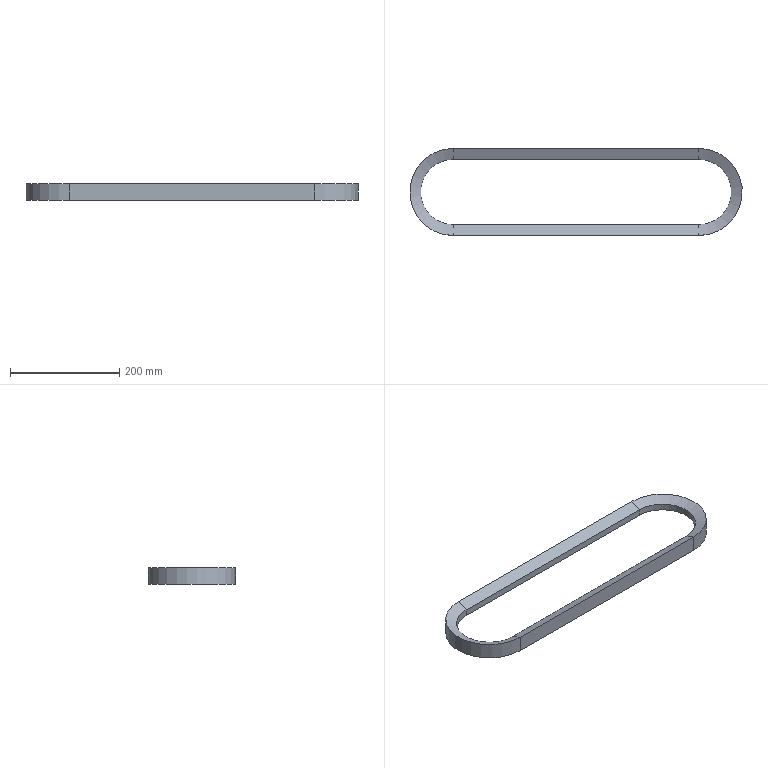Part | NX | 1 solid | 16 faces | box 610 x 160 x 30 mm | volume 573090 mm3 | plane 8 | cylinder 4 | cone 4 | commonest cylinder face diameters 120 x2 160 x2
STEP:
#1=CARTESIAN_POINT('',(450.,-80.,-15.));
#2=VERTEX_POINT('',#1);
#3=CARTESIAN_POINT('',(450.,-80.,15.));
#4=VERTEX_POINT('',#3);
#5=CARTESIAN_POINT('',(450.,-80.,-15.));
#6=DIRECTION('',(0.,0.,1.));
#7=VECTOR('',#6,1.);
#8=LINE('',#5,#7);
#9=EDGE_CURVE('',#2,#4,#8,.T.);
#10=ORIENTED_EDGE('',*,*,#9,.F.);
#11=CARTESIAN_POINT('',(450.,80.,-15.));
#12=VERTEX_POINT('',#11);
#13=CARTESIAN_POINT('',(450.,0.,-15.));
#14=DIRECTION('',(0.,0.,1.));
#15=DIRECTION('',(1.,0.,0.));
#16=AXIS2_PLACEMENT_3D('',#13,#14,#15);
#17=CIRCLE('',#16,80.);
#18=EDGE_CURVE('',#2,#12,#17,.T.);
#19=ORIENTED_EDGE('',*,*,#18,.T.);
#20=CARTESIAN_POINT('',(450.,80.,15.));
#21=VERTEX_POINT('',#20);
#22=CARTESIAN_POINT('',(450.,80.,-15.));
#23=DIRECTION('',(0.,0.,1.));
#24=VECTOR('',#23,1.);
#25=LINE('',#22,#24);
#26=EDGE_CURVE('',#12,#21,#25,.T.);
#27=ORIENTED_EDGE('',*,*,#26,.T.);
#28=CARTESIAN_POINT('',(450.,0.,15.));
#29=DIRECTION('',(0.,0.,1.));
#30=DIRECTION('',(1.,0.,0.));
#31=AXIS2_PLACEMENT_3D('',#28,#29,#30);
#32=CIRCLE('',#31,80.);
#33=EDGE_CURVE('',#4,#21,#32,.T.);
#34=ORIENTED_EDGE('',*,*,#33,.F.);
#35=EDGE_LOOP('',(#10,#19,#27,#34));
#36=FACE_OUTER_BOUND('',#35,.T.);
#37=CARTESIAN_POINT('',(450.,0.,0.));
#38=DIRECTION('',(0.,0.,1.));
#39=DIRECTION('',(1.,0.,0.));
#40=AXIS2_PLACEMENT_3D('',#37,#38,#39);
#41=CYLINDRICAL_SURFACE('',#40,80.);
#42=ADVANCED_FACE('',(#36),#41,.T.);
#43=CARTESIAN_POINT('',(450.,-60.,-6.25));
#44=VERTEX_POINT('',#43);
#45=CARTESIAN_POINT('',(450.,-60.,-6.25));
#46=DIRECTION('',(0.,-0.9162,-0.4008));
#47=VECTOR('',#46,1.);
#48=LINE('',#45,#47);
#49=EDGE_CURVE('',#44,#2,#48,.T.);
#50=ORIENTED_EDGE('',*,*,#49,.F.);
#51=CARTESIAN_POINT('',(450.,60.,-6.25));
#52=VERTEX_POINT('',#51);
#53=CARTESIAN_POINT('',(450.,0.,-6.25));
#54=DIRECTION('',(0.,0.,1.));
#55=DIRECTION('',(1.,0.,0.));
#56=AXIS2_PLACEMENT_3D('',#53,#54,#55);
#57=CIRCLE('',#56,60.);
#58=EDGE_CURVE('',#44,#52,#57,.T.);
#59=ORIENTED_EDGE('',*,*,#58,.T.);
#60=CARTESIAN_POINT('',(450.,60.,-6.25));
#61=DIRECTION('',(0.,0.9162,-0.4008));
#62=VECTOR('',#61,1.);
#63=LINE('',#60,#62);
#64=EDGE_CURVE('',#52,#12,#63,.T.);
#65=ORIENTED_EDGE('',*,*,#64,.T.);
#66=ORIENTED_EDGE('',*,*,#18,.F.);
#67=EDGE_LOOP('',(#50,#59,#65,#66));
#68=FACE_OUTER_BOUND('',#67,.T.);
#69=CARTESIAN_POINT('',(450.,0.,-6.25));
#70=DIRECTION('',(0.,0.,-1.));
#71=DIRECTION('',(-1.,0.,0.));
#72=AXIS2_PLACEMENT_3D('',#69,#70,#71);
#73=CONICAL_SURFACE('',#72,60.,66.371);
#74=ADVANCED_FACE('',(#68),#73,.F.);
#75=CARTESIAN_POINT('',(450.,-60.,6.25));
#76=VERTEX_POINT('',#75);
#77=CARTESIAN_POINT('',(450.,-60.,6.25));
#78=DIRECTION('',(0.,0.,-1.));
#79=VECTOR('',#78,1.);
#80=LINE('',#77,#79);
#81=EDGE_CURVE('',#76,#44,#80,.T.);
#82=ORIENTED_EDGE('',*,*,#81,.F.);
#83=CARTESIAN_POINT('',(450.,60.,6.25));
#84=VERTEX_POINT('',#83);
#85=CARTESIAN_POINT('',(450.,0.,6.25));
#86=DIRECTION('',(0.,0.,1.));
#87=DIRECTION('',(1.,0.,0.));
#88=AXIS2_PLACEMENT_3D('',#85,#86,#87);
#89=CIRCLE('',#88,60.);
#90=EDGE_CURVE('',#76,#84,#89,.T.);
#91=ORIENTED_EDGE('',*,*,#90,.T.);
#92=CARTESIAN_POINT('',(450.,60.,6.25));
#93=DIRECTION('',(0.,0.,-1.));
#94=VECTOR('',#93,1.);
#95=LINE('',#92,#94);
#96=EDGE_CURVE('',#84,#52,#95,.T.);
#97=ORIENTED_EDGE('',*,*,#96,.T.);
#98=ORIENTED_EDGE('',*,*,#58,.F.);
#99=EDGE_LOOP('',(#82,#91,#97,#98));
#100=FACE_OUTER_BOUND('',#99,.T.);
#101=CARTESIAN_POINT('',(450.,0.,0.));
#102=DIRECTION('',(0.,0.,1.));
#103=DIRECTION('',(1.,0.,0.));
#104=AXIS2_PLACEMENT_3D('',#101,#102,#103);
#105=CYLINDRICAL_SURFACE('',#104,60.);
#106=ADVANCED_FACE('',(#100),#105,.F.);
#107=CARTESIAN_POINT('',(450.,-80.,15.));
#108=DIRECTION('',(0.,0.9162,-0.4008));
#109=VECTOR('',#108,1.);
#110=LINE('',#107,#109);
#111=EDGE_CURVE('',#4,#76,#110,.T.);
#112=ORIENTED_EDGE('',*,*,#111,.F.);
#113=ORIENTED_EDGE('',*,*,#33,.T.);
#114=CARTESIAN_POINT('',(450.,80.,15.));
#115=DIRECTION('',(0.,-0.9162,-0.4008));
#116=VECTOR('',#115,1.);
#117=LINE('',#114,#116);
#118=EDGE_CURVE('',#21,#84,#117,.T.);
#119=ORIENTED_EDGE('',*,*,#118,.T.);
#120=ORIENTED_EDGE('',*,*,#90,.F.);
#121=EDGE_LOOP('',(#112,#113,#119,#120));
#122=FACE_OUTER_BOUND('',#121,.T.);
#123=CARTESIAN_POINT('',(450.,0.,15.));
#124=DIRECTION('',(0.,0.,1.));
#125=DIRECTION('',(1.,0.,0.));
#126=AXIS2_PLACEMENT_3D('',#123,#124,#125);
#127=CONICAL_SURFACE('',#126,80.,66.371);
#128=ADVANCED_FACE('',(#122),#127,.F.);
#129=CARTESIAN_POINT('',(0.,-80.,-15.));
#130=VERTEX_POINT('',#129);
#131=CARTESIAN_POINT('',(0.,-80.,15.));
#132=VERTEX_POINT('',#131);
#133=CARTESIAN_POINT('',(0.,-80.,-15.));
#134=DIRECTION('',(0.,0.,1.));
#135=VECTOR('',#134,1.);
#136=LINE('',#133,#135);
#137=EDGE_CURVE('',#130,#132,#136,.T.);
#138=ORIENTED_EDGE('',*,*,#137,.F.);
#139=CARTESIAN_POINT('',(0.,-80.,-15.));
#140=DIRECTION('',(1.,0.,0.));
#141=VECTOR('',#140,1.);
#142=LINE('',#139,#141);
#143=EDGE_CURVE('',#130,#2,#142,.T.);
#144=ORIENTED_EDGE('',*,*,#143,.T.);
#145=ORIENTED_EDGE('',*,*,#9,.T.);
#146=CARTESIAN_POINT('',(0.,-80.,15.));
#147=DIRECTION('',(1.,0.,0.));
#148=VECTOR('',#147,1.);
#149=LINE('',#146,#148);
#150=EDGE_CURVE('',#132,#4,#149,.T.);
#151=ORIENTED_EDGE('',*,*,#150,.F.);
#152=EDGE_LOOP('',(#138,#144,#145,#151));
#153=FACE_OUTER_BOUND('',#152,.T.);
#154=CARTESIAN_POINT('',(0.,-80.,-15.));
#155=DIRECTION('',(0.,1.,0.));
#156=DIRECTION('',(0.,0.,1.));
#157=AXIS2_PLACEMENT_3D('',#154,#155,#156);
#158=PLANE('',#157);
#159=ADVANCED_FACE('',(#153),#158,.F.);
#160=CARTESIAN_POINT('',(0.,-60.,-6.25));
#161=VERTEX_POINT('',#160);
#162=CARTESIAN_POINT('',(0.,-60.,-6.25));
#163=DIRECTION('',(0.,-0.9162,-0.4008));
#164=VECTOR('',#163,1.);
#165=LINE('',#162,#164);
#166=EDGE_CURVE('',#161,#130,#165,.T.);
#167=ORIENTED_EDGE('',*,*,#166,.F.);
#168=CARTESIAN_POINT('',(0.,-60.,-6.25));
#169=DIRECTION('',(1.,0.,0.));
#170=VECTOR('',#169,1.);
#171=LINE('',#168,#170);
#172=EDGE_CURVE('',#161,#44,#171,.T.);
#173=ORIENTED_EDGE('',*,*,#172,.T.);
#174=ORIENTED_EDGE('',*,*,#49,.T.);
#175=ORIENTED_EDGE('',*,*,#143,.F.);
#176=EDGE_LOOP('',(#167,#173,#174,#175));
#177=FACE_OUTER_BOUND('',#176,.T.);
#178=CARTESIAN_POINT('',(0.,-60.,-6.25));
#179=DIRECTION('',(0.,-0.4008,0.9162));
#180=DIRECTION('',(0.,-0.9162,-0.4008));
#181=AXIS2_PLACEMENT_3D('',#178,#179,#180);
#182=PLANE('',#181);
#183=ADVANCED_FACE('',(#177),#182,.F.);
#184=CARTESIAN_POINT('',(0.,-60.,6.25));
#185=VERTEX_POINT('',#184);
#186=CARTESIAN_POINT('',(0.,-60.,6.25));
#187=DIRECTION('',(0.,0.,-1.));
#188=VECTOR('',#187,1.);
#189=LINE('',#186,#188);
#190=EDGE_CURVE('',#185,#161,#189,.T.);
#191=ORIENTED_EDGE('',*,*,#190,.F.);
#192=CARTESIAN_POINT('',(0.,-60.,6.25));
#193=DIRECTION('',(1.,0.,0.));
#194=VECTOR('',#193,1.);
#195=LINE('',#192,#194);
#196=EDGE_CURVE('',#185,#76,#195,.T.);
#197=ORIENTED_EDGE('',*,*,#196,.T.);
#198=ORIENTED_EDGE('',*,*,#81,.T.);
#199=ORIENTED_EDGE('',*,*,#172,.F.);
#200=EDGE_LOOP('',(#191,#197,#198,#199));
#201=FACE_OUTER_BOUND('',#200,.T.);
#202=CARTESIAN_POINT('',(0.,-60.,6.25));
#203=DIRECTION('',(0.,-1.,0.));
#204=DIRECTION('',(0.,0.,-1.));
#205=AXIS2_PLACEMENT_3D('',#202,#203,#204);
#206=PLANE('',#205);
#207=ADVANCED_FACE('',(#201),#206,.F.);
#208=CARTESIAN_POINT('',(0.,-80.,15.));
#209=DIRECTION('',(0.,0.9162,-0.4008));
#210=VECTOR('',#209,1.);
#211=LINE('',#208,#210);
#212=EDGE_CURVE('',#132,#185,#211,.T.);
#213=ORIENTED_EDGE('',*,*,#212,.F.);
#214=ORIENTED_EDGE('',*,*,#150,.T.);
#215=ORIENTED_EDGE('',*,*,#111,.T.);
#216=ORIENTED_EDGE('',*,*,#196,.F.);
#217=EDGE_LOOP('',(#213,#214,#215,#216));
#218=FACE_OUTER_BOUND('',#217,.T.);
#219=CARTESIAN_POINT('',(0.,-80.,15.));
#220=DIRECTION('',(0.,-0.4008,-0.9162));
#221=DIRECTION('',(0.,0.9162,-0.4008));
#222=AXIS2_PLACEMENT_3D('',#219,#220,#221);
#223=PLANE('',#222);
#224=ADVANCED_FACE('',(#218),#223,.F.);
#225=CARTESIAN_POINT('',(0.,60.,6.25));
#226=VERTEX_POINT('',#225);
#227=CARTESIAN_POINT('',(0.,0.,6.25));
#228=DIRECTION('',(0.,0.,-1.));
#229=DIRECTION('',(-1.,0.,0.));
#230=AXIS2_PLACEMENT_3D('',#227,#228,#229);
#231=CIRCLE('',#230,60.);
#232=EDGE_CURVE('',#185,#226,#231,.T.);
#233=ORIENTED_EDGE('',*,*,#232,.T.);
#234=CARTESIAN_POINT('',(0.,80.,15.));
#235=VERTEX_POINT('',#234);
#236=CARTESIAN_POINT('',(0.,80.,15.));
#237=DIRECTION('',(0.,-0.9162,-0.4008));
#238=VECTOR('',#237,1.);
#239=LINE('',#236,#238);
#240=EDGE_CURVE('',#235,#226,#239,.T.);
#241=ORIENTED_EDGE('',*,*,#240,.F.);
#242=CARTESIAN_POINT('',(0.,0.,15.));
#243=DIRECTION('',(0.,0.,-1.));
#244=DIRECTION('',(-1.,0.,0.));
#245=AXIS2_PLACEMENT_3D('',#242,#243,#244);
#246=CIRCLE('',#245,80.);
#247=EDGE_CURVE('',#132,#235,#246,.T.);
#248=ORIENTED_EDGE('',*,*,#247,.F.);
#249=ORIENTED_EDGE('',*,*,#212,.T.);
#250=EDGE_LOOP('',(#233,#241,#248,#249));
#251=FACE_OUTER_BOUND('',#250,.T.);
#252=CARTESIAN_POINT('',(0.,0.,15.));
#253=DIRECTION('',(0.,0.,1.));
#254=DIRECTION('',(1.,0.,0.));
#255=AXIS2_PLACEMENT_3D('',#252,#253,#254);
#256=CONICAL_SURFACE('',#255,80.,66.371);
#257=ADVANCED_FACE('',(#251),#256,.F.);
#258=CARTESIAN_POINT('',(0.,60.,-6.25));
#259=VERTEX_POINT('',#258);
#260=CARTESIAN_POINT('',(0.,0.,-6.25));
#261=DIRECTION('',(0.,0.,-1.));
#262=DIRECTION('',(-1.,0.,0.));
#263=AXIS2_PLACEMENT_3D('',#260,#261,#262);
#264=CIRCLE('',#263,60.);
#265=EDGE_CURVE('',#161,#259,#264,.T.);
#266=ORIENTED_EDGE('',*,*,#265,.T.);
#267=CARTESIAN_POINT('',(0.,60.,6.25));
#268=DIRECTION('',(0.,0.,-1.));
#269=VECTOR('',#268,1.);
#270=LINE('',#267,#269);
#271=EDGE_CURVE('',#226,#259,#270,.T.);
#272=ORIENTED_EDGE('',*,*,#271,.F.);
#273=ORIENTED_EDGE('',*,*,#232,.F.);
#274=ORIENTED_EDGE('',*,*,#190,.T.);
#275=EDGE_LOOP('',(#266,#272,#273,#274));
#276=FACE_OUTER_BOUND('',#275,.T.);
#277=CARTESIAN_POINT('',(0.,0.,0.));
#278=DIRECTION('',(0.,0.,-1.));
#279=DIRECTION('',(-1.,0.,0.));
#280=AXIS2_PLACEMENT_3D('',#277,#278,#279);
#281=CYLINDRICAL_SURFACE('',#280,60.);
#282=ADVANCED_FACE('',(#276),#281,.F.);
#283=CARTESIAN_POINT('',(0.,80.,-15.));
#284=VERTEX_POINT('',#283);
#285=CARTESIAN_POINT('',(0.,0.,-15.));
#286=DIRECTION('',(0.,0.,-1.));
#287=DIRECTION('',(-1.,0.,0.));
#288=AXIS2_PLACEMENT_3D('',#285,#286,#287);
#289=CIRCLE('',#288,80.);
#290=EDGE_CURVE('',#130,#284,#289,.T.);
#291=ORIENTED_EDGE('',*,*,#290,.T.);
#292=CARTESIAN_POINT('',(0.,60.,-6.25));
#293=DIRECTION('',(0.,0.9162,-0.4008));
#294=VECTOR('',#293,1.);
#295=LINE('',#292,#294);
#296=EDGE_CURVE('',#259,#284,#295,.T.);
#297=ORIENTED_EDGE('',*,*,#296,.F.);
#298=ORIENTED_EDGE('',*,*,#265,.F.);
#299=ORIENTED_EDGE('',*,*,#166,.T.);
#300=EDGE_LOOP('',(#291,#297,#298,#299));
#301=FACE_OUTER_BOUND('',#300,.T.);
#302=CARTESIAN_POINT('',(0.,0.,-6.25));
#303=DIRECTION('',(0.,0.,-1.));
#304=DIRECTION('',(-1.,0.,0.));
#305=AXIS2_PLACEMENT_3D('',#302,#303,#304);
#306=CONICAL_SURFACE('',#305,60.,66.371);
#307=ADVANCED_FACE('',(#301),#306,.F.);
#308=ORIENTED_EDGE('',*,*,#137,.T.);
#309=ORIENTED_EDGE('',*,*,#247,.T.);
#310=CARTESIAN_POINT('',(0.,80.,-15.));
#311=DIRECTION('',(0.,0.,1.));
#312=VECTOR('',#311,1.);
#313=LINE('',#310,#312);
#314=EDGE_CURVE('',#284,#235,#313,.T.);
#315=ORIENTED_EDGE('',*,*,#314,.F.);
#316=ORIENTED_EDGE('',*,*,#290,.F.);
#317=EDGE_LOOP('',(#308,#309,#315,#316));
#318=FACE_OUTER_BOUND('',#317,.T.);
#319=CARTESIAN_POINT('',(0.,0.,0.));
#320=DIRECTION('',(0.,0.,-1.));
#321=DIRECTION('',(-1.,0.,0.));
#322=AXIS2_PLACEMENT_3D('',#319,#320,#321);
#323=CYLINDRICAL_SURFACE('',#322,80.);
#324=ADVANCED_FACE('',(#318),#323,.T.);
#325=ORIENTED_EDGE('',*,*,#118,.F.);
#326=CARTESIAN_POINT('',(0.,80.,15.));
#327=DIRECTION('',(1.,0.,0.));
#328=VECTOR('',#327,1.);
#329=LINE('',#326,#328);
#330=EDGE_CURVE('',#235,#21,#329,.T.);
#331=ORIENTED_EDGE('',*,*,#330,.F.);
#332=ORIENTED_EDGE('',*,*,#240,.T.);
#333=CARTESIAN_POINT('',(0.,60.,6.25));
#334=DIRECTION('',(1.,0.,0.));
#335=VECTOR('',#334,1.);
#336=LINE('',#333,#335);
#337=EDGE_CURVE('',#226,#84,#336,.T.);
#338=ORIENTED_EDGE('',*,*,#337,.T.);
#339=EDGE_LOOP('',(#325,#331,#332,#338));
#340=FACE_OUTER_BOUND('',#339,.T.);
#341=CARTESIAN_POINT('',(0.,80.,15.));
#342=DIRECTION('',(0.,-0.4008,0.9162));
#343=DIRECTION('',(0.,-0.9162,-0.4008));
#344=AXIS2_PLACEMENT_3D('',#341,#342,#343);
#345=PLANE('',#344);
#346=ADVANCED_FACE('',(#340),#345,.T.);
#347=ORIENTED_EDGE('',*,*,#26,.F.);
#348=CARTESIAN_POINT('',(0.,80.,-15.));
#349=DIRECTION('',(1.,0.,0.));
#350=VECTOR('',#349,1.);
#351=LINE('',#348,#350);
#352=EDGE_CURVE('',#284,#12,#351,.T.);
#353=ORIENTED_EDGE('',*,*,#352,.F.);
#354=ORIENTED_EDGE('',*,*,#314,.T.);
#355=ORIENTED_EDGE('',*,*,#330,.T.);
#356=EDGE_LOOP('',(#347,#353,#354,#355));
#357=FACE_OUTER_BOUND('',#356,.T.);
#358=CARTESIAN_POINT('',(0.,80.,-15.));
#359=DIRECTION('',(0.,1.,0.));
#360=DIRECTION('',(0.,0.,1.));
#361=AXIS2_PLACEMENT_3D('',#358,#359,#360);
#362=PLANE('',#361);
#363=ADVANCED_FACE('',(#357),#362,.T.);
#364=ORIENTED_EDGE('',*,*,#64,.F.);
#365=CARTESIAN_POINT('',(0.,60.,-6.25));
#366=DIRECTION('',(1.,0.,0.));
#367=VECTOR('',#366,1.);
#368=LINE('',#365,#367);
#369=EDGE_CURVE('',#259,#52,#368,.T.);
#370=ORIENTED_EDGE('',*,*,#369,.F.);
#371=ORIENTED_EDGE('',*,*,#296,.T.);
#372=ORIENTED_EDGE('',*,*,#352,.T.);
#373=EDGE_LOOP('',(#364,#370,#371,#372));
#374=FACE_OUTER_BOUND('',#373,.T.);
#375=CARTESIAN_POINT('',(0.,60.,-6.25));
#376=DIRECTION('',(0.,-0.4008,-0.9162));
#377=DIRECTION('',(0.,0.9162,-0.4008));
#378=AXIS2_PLACEMENT_3D('',#375,#376,#377);
#379=PLANE('',#378);
#380=ADVANCED_FACE('',(#374),#379,.T.);
#381=ORIENTED_EDGE('',*,*,#96,.F.);
#382=ORIENTED_EDGE('',*,*,#337,.F.);
#383=ORIENTED_EDGE('',*,*,#271,.T.);
#384=ORIENTED_EDGE('',*,*,#369,.T.);
#385=EDGE_LOOP('',(#381,#382,#383,#384));
#386=FACE_OUTER_BOUND('',#385,.T.);
#387=CARTESIAN_POINT('',(0.,60.,6.25));
#388=DIRECTION('',(0.,-1.,0.));
#389=DIRECTION('',(0.,0.,-1.));
#390=AXIS2_PLACEMENT_3D('',#387,#388,#389);
#391=PLANE('',#390);
#392=ADVANCED_FACE('',(#386),#391,.T.);
#393=CLOSED_SHELL('',(#42,#74,#106,#128,#159,#183,#207,#224,#257,#282,#307,#324,#346,#363,#380,#392));
#394=MANIFOLD_SOLID_BREP('',#393);
#395=(LENGTH_UNIT()NAMED_UNIT(*)SI_UNIT(.MILLI.,.METRE.));
#396=UNCERTAINTY_MEASURE_WITH_UNIT(LENGTH_MEASURE(0.00002),#395,'','');
#397=(NAMED_UNIT(*)PLANE_ANGLE_UNIT()SI_UNIT($,.RADIAN.));
#398=PLANE_ANGLE_MEASURE_WITH_UNIT(PLANE_ANGLE_MEASURE(0.01745),#397);
#399=DIMENSIONAL_EXPONENTS(0.,0.,0.,0.,0.,0.,0.);
#400=(CONVERSION_BASED_UNIT('DEGREE',#398)NAMED_UNIT(#399)PLANE_ANGLE_UNIT());
#401=(NAMED_UNIT(*)SI_UNIT($,.STERADIAN.)SOLID_ANGLE_UNIT());
#402=(GEOMETRIC_REPRESENTATION_CONTEXT(3)GLOBAL_UNCERTAINTY_ASSIGNED_CONTEXT((#396))GLOBAL_UNIT_ASSIGNED_CONTEXT((#395,#400,#401))REPRESENTATION_CONTEXT('',''));
#403=ADVANCED_BREP_SHAPE_REPRESENTATION('',(#394),#402);